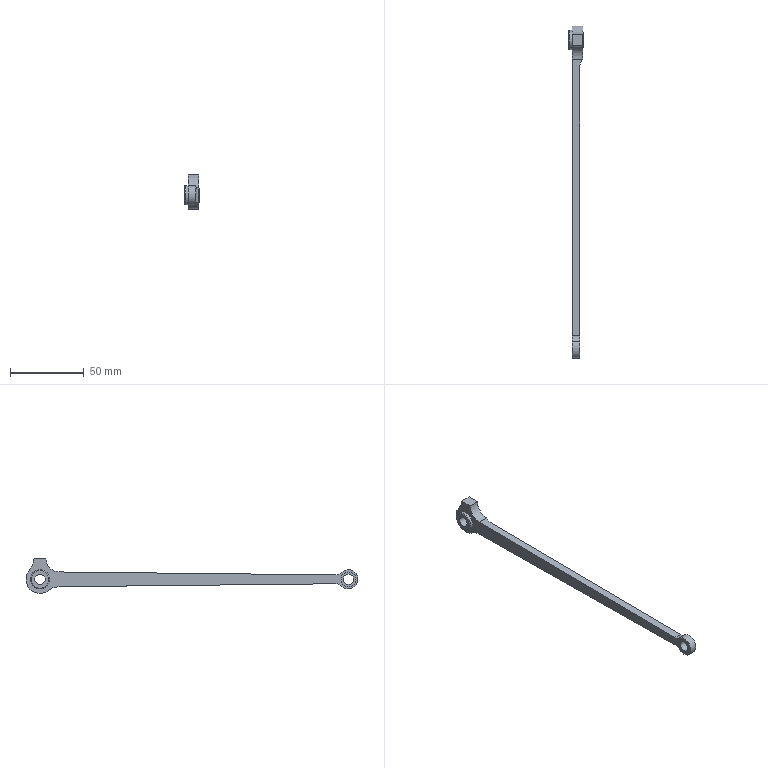Part | STEP file | 2-07 | 3 solids | 36 faces | box 10 x 225 x 23.5 mm | volume 9355 mm3 | cylinder 19 | plane 16 | torus 1 | commonest cylinder face diameters 1 x4 10 x4 7 x2 12 x2 13 x2 16 x1